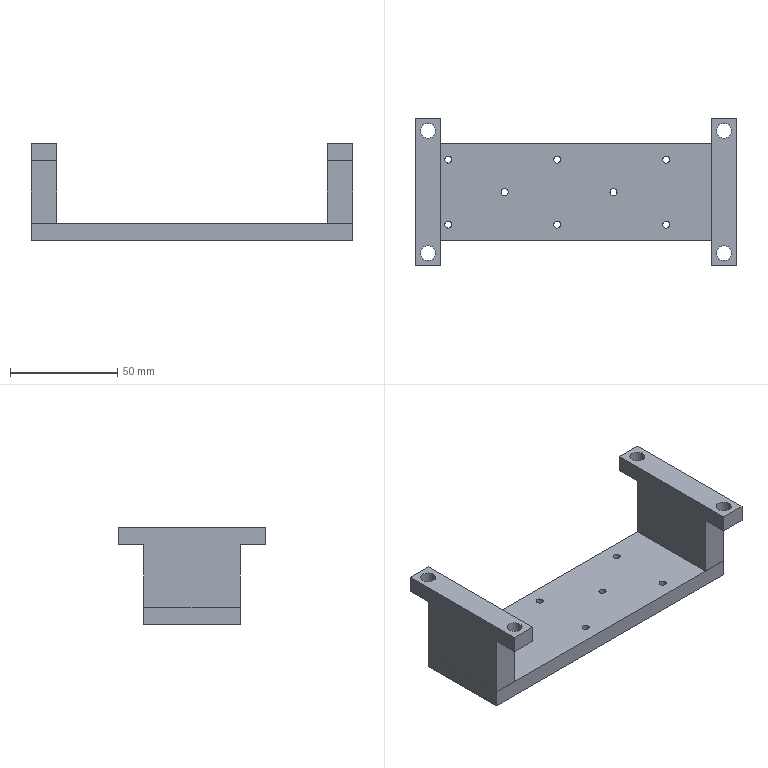Part | STEP file | Cylinder mounting plate_default<machined> | 3 solids | 88 faces | box 150 x 69 x 45 mm | volume 93928 mm3 | cylinder 50 | plane 30 | cone 8 | commonest cylinder face diameters 3.3 x18 4.2 x8 5.3 x8 7 x8 10 x8